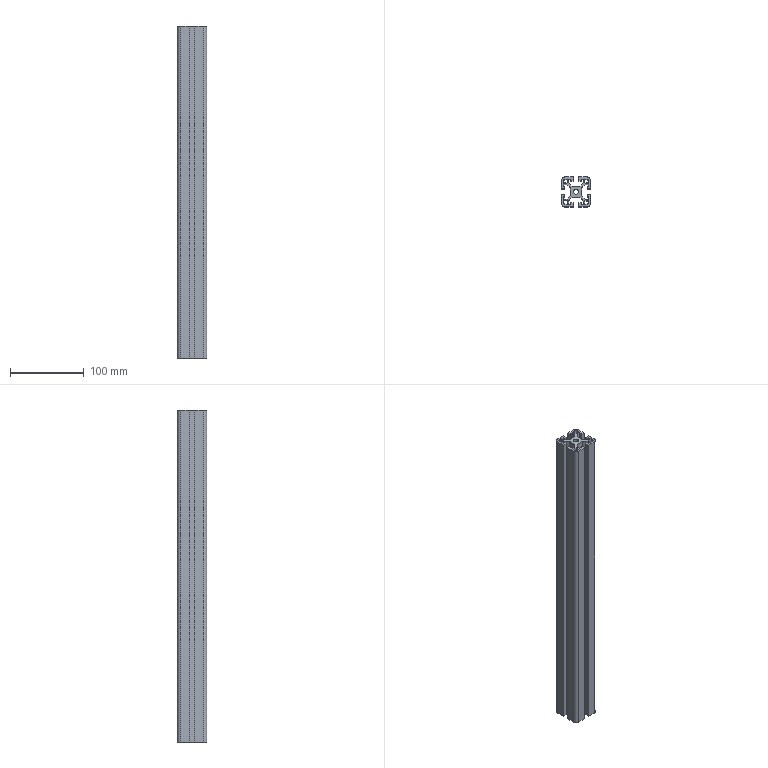Part | STEP file | 4040-450 | 1 solid | 88 faces | box 40 x 40 x 450 mm | volume 316776 mm3 | plane 78 | cylinder 10 | commonest cylinder face diameters 4 x4 10 x4 6.8 x2